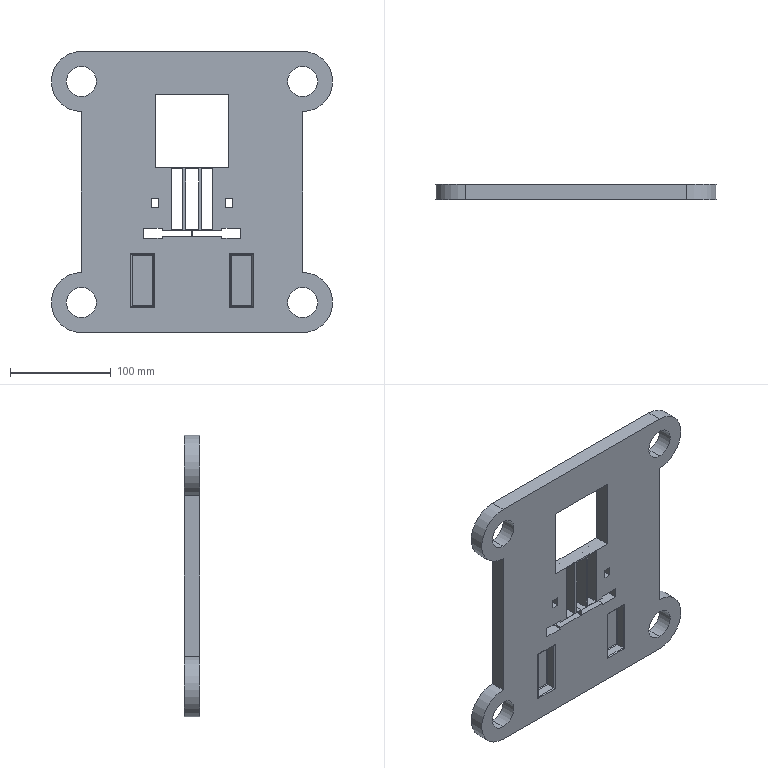Part | SolidWorks | features Cut 2, Extrusion 1, Fillet 1, MirrorPattern 1 | 1 solid | 84 faces | box 280 x 15 x 280 mm | volume 817644 mm3 | plane 56 | cylinder 28 | commonest cylinder face diameters 2 x16 30 x8 60 x4